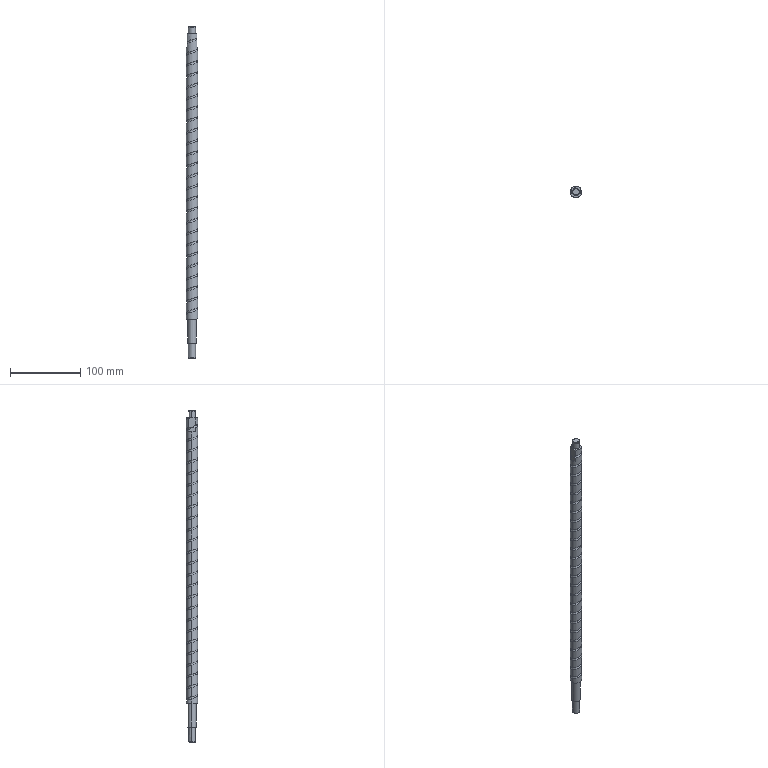Part | STEP file | Screw rod BLK1616-3.6G0+472 | 1 solid | 87 faces | box 16 x 16 x 472 mm | volume 82941 mm3 | cylinder 65 | plane 16 | cone 5 | spline 1 | commonest cylinder face diameters 16 x54 10 x4 9 x2 9.6 x2 12 x2 3 x1